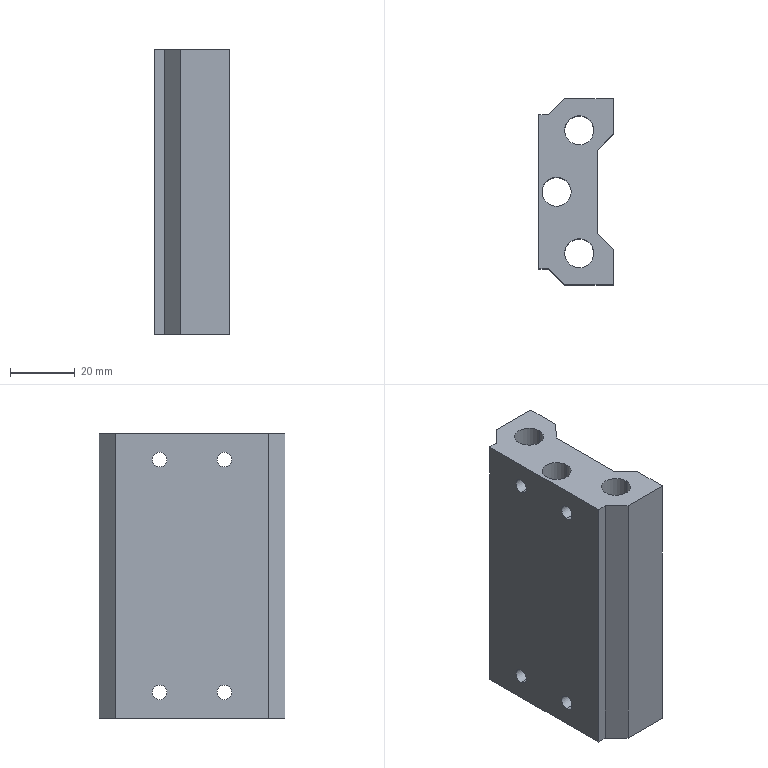Part | STEP file | Solenoid valve base 7V100M4F | 1 solid | 28 faces | box 23 x 57.5 x 88 mm | volume 80180 mm3 | cylinder 14 | plane 14 | commonest cylinder face diameters 4.5 x8 9 x6